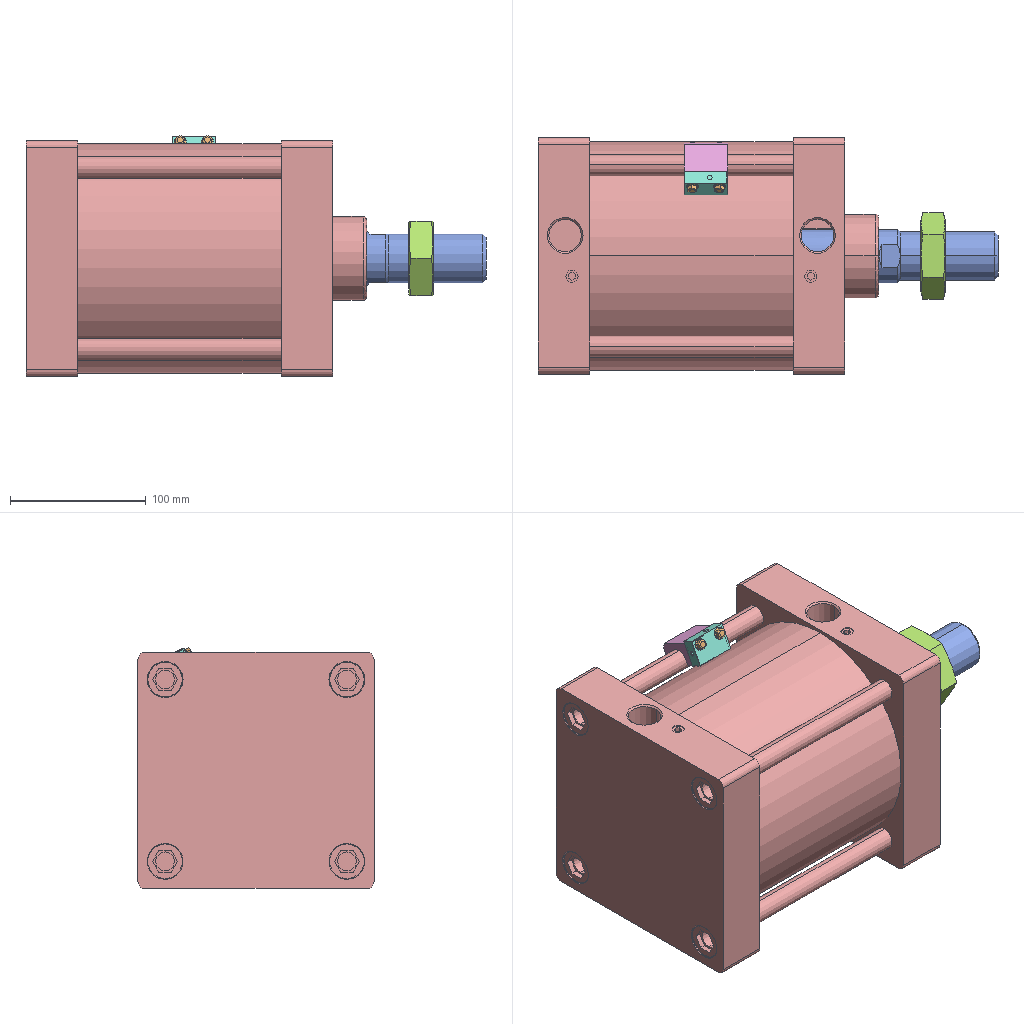Assembly | SolidWorks | 7 different items | 10 placed | box 339 x 174 x 178 mm
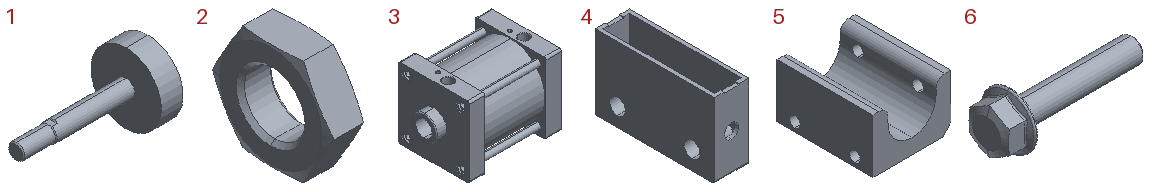Parts list (item | name | quantity | size | volume | features):
1 | - | x1 | 301 x 160 x 160 mm | 1302352 mm3 | features BaseBody 1
2 | - | x1 | 18 x 63.509 x 55 mm | 32144 mm3 | features BaseBody 1
3 | - | x1 | 251 x 174 x 174 mm | 2665389 mm3 | features BaseBody 1
4 | - | x1 | 9.2 x 32 x 20.1 mm | 1950 mm3 | features ICE 8, Fillet 2, Extrusion 1
5 | - | x1 | 26 x 32 x 18 mm | 8652 mm3 | features ICE 3, Extrusion 1
6 | - | x4 | 24.05 x 9 x 9 mm | 413.187 mm3 | features BaseBody 1, Scale 1
7 | Locating Pin | x1 | - | - | -
Mates (type | each side: item.copy, entity, surface, feature):
Concentric | 3.1 face cylinder Input1 | 5.1 face cylinder Boss-Extrude1
Coincident | 5.1 face plane Boss-Extrude1 | 4.1 face plane Boss-Extrude1 | 2 times
Tangent | 3.1 face cylinder Input1 | 4.1 face plane Boss-Extrude1
Concentric | 5.1 face cylinder Cut-Extrude3 | 4.1 face cylinder Cut-Extrude1 | 2 times
Concentric | 5.1 face cylinder Cut-Extrude1 | 6.1 face cylinder Input1
Coincident | 5.1 face plane Boss-Extrude1 | 6.1 face plane Input1
Concentric | 5.1 face cylinder Cut-Extrude1 | 6.2 face cylinder Input1
Coincident | 5.1 face plane Boss-Extrude1 | 6.2 face plane Input1
Concentric | 4.1 face cylinder Cut-Extrude1 | 6.3 face cylinder Input1
Coincident | 4.1 face plane Boss-Extrude1 | 6.3 face plane Input1
Concentric | 4.1 face cylinder Cut-Extrude1 | 6.4 face cylinder Input1
Coincident | 4.1 face plane Boss-Extrude1 | 6.4 face plane Input1